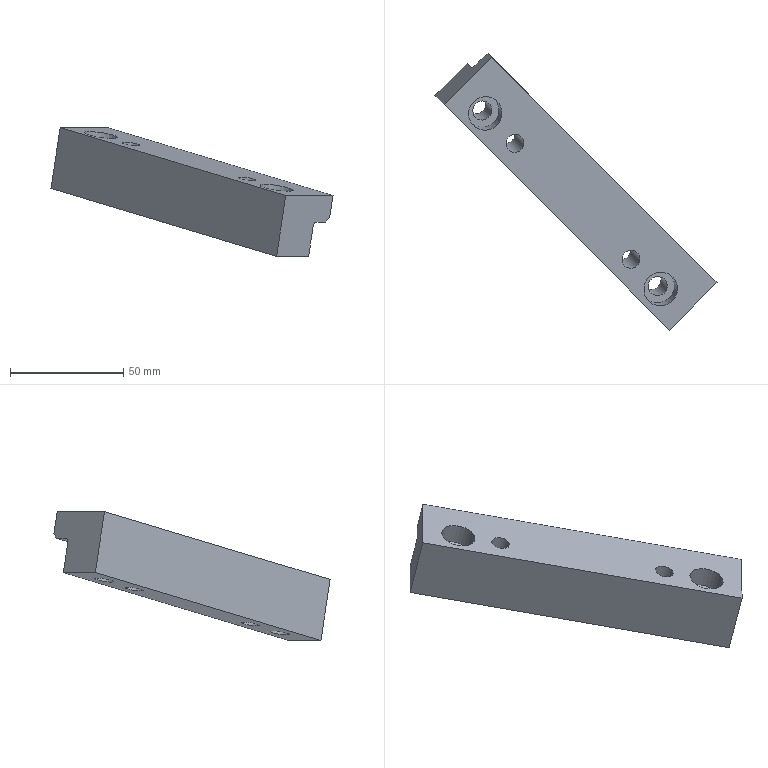Part | STEP file | gslz 2016.10.28-13_id1550_x_t | 1 solid | 18 faces | box 124.501 x 121.928 x 56.838 mm | volume 87407 mm3 | plane 11 | cylinder 7 | commonest cylinder face diameters 8 x2 8.5 x2 15 x2 4 x1